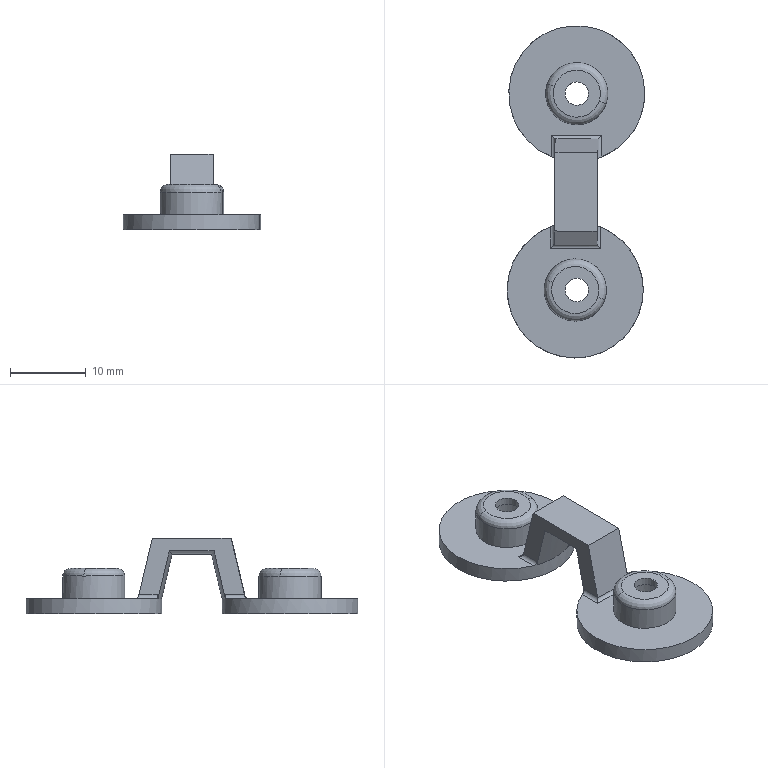Part | STEP file | Wytnij-wyci_gni_cie3_1 | 1 solid | 38 faces | box 18.204 x 43.999 x 10 mm | volume 1454 mm3 | cylinder 14 | plane 13 | spline 11 | commonest cylinder face diameters 1 x6 3.1 x2 6.05 x2 8.24 x2 18 x2